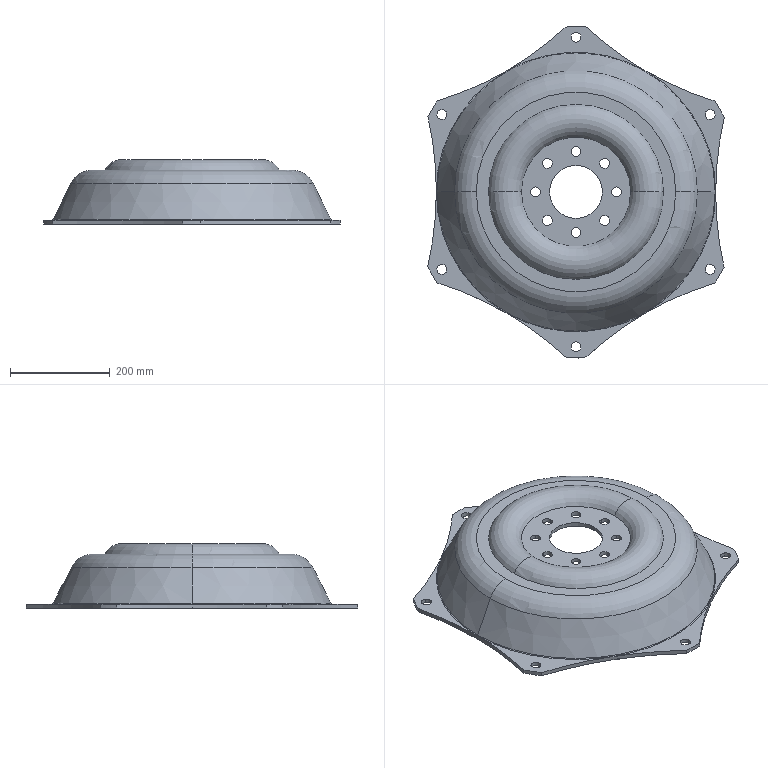Part | SolidWorks | 1 solid | 74 faces | box 593.907 x 665 x 128.5 mm | volume 2994623 mm3 | cylinder 42 | plane 16 | torus 12 | cone 4 | commonest cylinder face diameters 20 x28 665 x6 1339 x6 106 x2